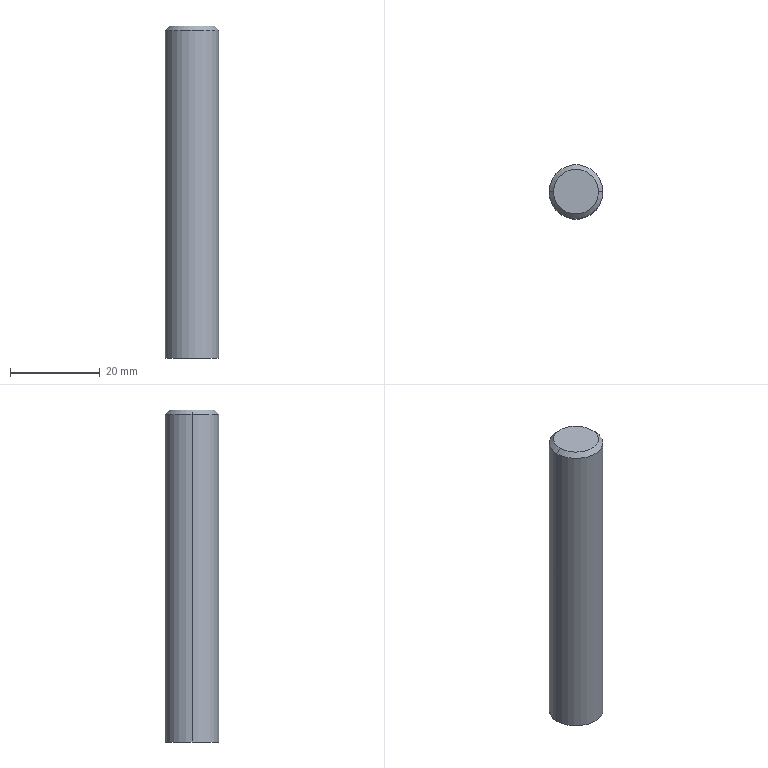Part | 1 solid | 15 faces | box 12 x 12 x 74 mm | volume 7564 mm3 | cone 6 | cylinder 6 | plane 3 | commonest cylinder face diameters 5 x2 8 x2 12 x2
STEP:
#1=CARTESIAN_POINT('',(2.5,0.,8.55));
#2=VERTEX_POINT('',#1);
#3=CARTESIAN_POINT('',(-2.5,0.,8.55));
#4=VERTEX_POINT('',#3);
#5=CARTESIAN_POINT('',(0.,0.,8.55));
#6=DIRECTION('',(0.,0.,-1.));
#7=DIRECTION('',(-1.,0.,0.));
#8=AXIS2_PLACEMENT_3D('',#5,#6,#7);
#9=CIRCLE('',#8,2.5);
#10=EDGE_CURVE('',#2,#4,#9,.T.);
#11=ORIENTED_EDGE('',*,*,#10,.F.);
#12=CARTESIAN_POINT('',(3.05,0.,8.));
#13=VERTEX_POINT('',#12);
#14=CARTESIAN_POINT('',(3.05,0.,8.));
#15=DIRECTION('',(0.7071,0.,-0.7071));
#16=VECTOR('',#15,1000.);
#17=LINE('',#14,#16);
#18=EDGE_CURVE('',#2,#13,#17,.T.);
#19=ORIENTED_EDGE('',*,*,#18,.T.);
#20=CARTESIAN_POINT('',(-3.05,0.,8.));
#21=VERTEX_POINT('',#20);
#22=CARTESIAN_POINT('',(0.,0.,8.));
#23=DIRECTION('',(0.,0.,-1.));
#24=DIRECTION('',(-1.,0.,0.));
#25=AXIS2_PLACEMENT_3D('',#22,#23,#24);
#26=CIRCLE('',#25,3.05);
#27=EDGE_CURVE('',#13,#21,#26,.T.);
#28=ORIENTED_EDGE('',*,*,#27,.T.);
#29=CARTESIAN_POINT('',(-3.05,0.,8.));
#30=DIRECTION('',(-0.7071,0.,-0.7071));
#31=VECTOR('',#30,1000.);
#32=LINE('',#29,#31);
#33=EDGE_CURVE('',#4,#21,#32,.T.);
#34=ORIENTED_EDGE('',*,*,#33,.F.);
#35=EDGE_LOOP('',(#11,#19,#28,#34));
#36=FACE_OUTER_BOUND('',#35,.T.);
#37=CARTESIAN_POINT('',(0.,0.,8.));
#38=DIRECTION('',(0.,0.,-1.));
#39=DIRECTION('',(-1.,0.,0.));
#40=AXIS2_PLACEMENT_3D('',#37,#38,#39);
#41=CONICAL_SURFACE('',#40,3.05,0.7854);
#42=ADVANCED_FACE('',(#36),#41,.F.);
#43=CARTESIAN_POINT('',(2.5,0.,27.));
#44=VERTEX_POINT('',#43);
#45=CARTESIAN_POINT('',(-2.5,0.,27.));
#46=VERTEX_POINT('',#45);
#47=CARTESIAN_POINT('',(0.,0.,27.));
#48=DIRECTION('',(0.,0.,-1.));
#49=DIRECTION('',(-1.,0.,0.));
#50=AXIS2_PLACEMENT_3D('',#47,#48,#49);
#51=CIRCLE('',#50,2.5);
#52=EDGE_CURVE('',#44,#46,#51,.T.);
#53=ORIENTED_EDGE('',*,*,#52,.F.);
#54=CARTESIAN_POINT('',(2.5,0.,8.));
#55=DIRECTION('',(0.,0.,-1.));
#56=VECTOR('',#55,1000.);
#57=LINE('',#54,#56);
#58=EDGE_CURVE('',#44,#2,#57,.T.);
#59=ORIENTED_EDGE('',*,*,#58,.T.);
#60=ORIENTED_EDGE('',*,*,#10,.T.);
#61=CARTESIAN_POINT('',(-2.5,0.,8.));
#62=DIRECTION('',(0.,0.,-1.));
#63=VECTOR('',#62,1000.);
#64=LINE('',#61,#63);
#65=EDGE_CURVE('',#46,#4,#64,.T.);
#66=ORIENTED_EDGE('',*,*,#65,.F.);
#67=EDGE_LOOP('',(#53,#59,#60,#66));
#68=FACE_OUTER_BOUND('',#67,.T.);
#69=CARTESIAN_POINT('',(0.,0.,8.));
#70=DIRECTION('',(0.,0.,-1.));
#71=DIRECTION('',(-1.,0.,0.));
#72=AXIS2_PLACEMENT_3D('',#69,#70,#71);
#73=CYLINDRICAL_SURFACE('',#72,2.5);
#74=ADVANCED_FACE('',(#68),#73,.F.);
#75=CARTESIAN_POINT('',(0.,0.,28.502));
#76=VERTEX_POINT('',#75);
#77=CARTESIAN_POINT('',(-2.5,0.,27.));
#78=DIRECTION('',(-0.8572,0.,-0.515));
#79=VECTOR('',#78,1000.);
#80=LINE('',#77,#79);
#81=EDGE_CURVE('',#76,#46,#80,.T.);
#82=ORIENTED_EDGE('',*,*,#81,.F.);
#83=CARTESIAN_POINT('',(2.5,0.,27.));
#84=DIRECTION('',(0.8572,0.,-0.515));
#85=VECTOR('',#84,1000.);
#86=LINE('',#83,#85);
#87=EDGE_CURVE('',#76,#44,#86,.T.);
#88=ORIENTED_EDGE('',*,*,#87,.T.);
#89=ORIENTED_EDGE('',*,*,#52,.T.);
#90=EDGE_LOOP('',(#82,#88,#89));
#91=FACE_OUTER_BOUND('',#90,.T.);
#92=CARTESIAN_POINT('',(0.,0.,27.));
#93=DIRECTION('',(0.,0.,-1.));
#94=DIRECTION('',(-1.,0.,0.));
#95=AXIS2_PLACEMENT_3D('',#92,#93,#94);
#96=CONICAL_SURFACE('',#95,2.5,1.03);
#97=ADVANCED_FACE('',(#91),#96,.F.);
#98=CARTESIAN_POINT('',(4.,0.,8.));
#99=VERTEX_POINT('',#98);
#100=CARTESIAN_POINT('',(-4.,0.,8.));
#101=VERTEX_POINT('',#100);
#102=CARTESIAN_POINT('',(0.,0.,8.));
#103=DIRECTION('',(0.,0.,-1.));
#104=DIRECTION('',(-1.,0.,0.));
#105=AXIS2_PLACEMENT_3D('',#102,#103,#104);
#106=CIRCLE('',#105,4.);
#107=EDGE_CURVE('',#99,#101,#106,.T.);
#108=ORIENTED_EDGE('',*,*,#107,.F.);
#109=CARTESIAN_POINT('',(4.,0.,0.));
#110=VERTEX_POINT('',#109);
#111=CARTESIAN_POINT('',(4.,0.,8.));
#112=DIRECTION('',(0.,0.,-1.));
#113=VECTOR('',#112,1000.);
#114=LINE('',#111,#113);
#115=EDGE_CURVE('',#99,#110,#114,.T.);
#116=ORIENTED_EDGE('',*,*,#115,.T.);
#117=CARTESIAN_POINT('',(-4.,0.,0.));
#118=VERTEX_POINT('',#117);
#119=CARTESIAN_POINT('',(0.,0.,0.));
#120=DIRECTION('',(0.,0.,-1.));
#121=DIRECTION('',(-1.,0.,0.));
#122=AXIS2_PLACEMENT_3D('',#119,#120,#121);
#123=CIRCLE('',#122,4.);
#124=EDGE_CURVE('',#110,#118,#123,.T.);
#125=ORIENTED_EDGE('',*,*,#124,.T.);
#126=CARTESIAN_POINT('',(-4.,0.,8.));
#127=DIRECTION('',(0.,0.,-1.));
#128=VECTOR('',#127,1000.);
#129=LINE('',#126,#128);
#130=EDGE_CURVE('',#101,#118,#129,.T.);
#131=ORIENTED_EDGE('',*,*,#130,.F.);
#132=EDGE_LOOP('',(#108,#116,#125,#131));
#133=FACE_OUTER_BOUND('',#132,.T.);
#134=CARTESIAN_POINT('',(0.,0.,8.));
#135=DIRECTION('',(0.,0.,-1.));
#136=DIRECTION('',(-1.,0.,0.));
#137=AXIS2_PLACEMENT_3D('',#134,#135,#136);
#138=CYLINDRICAL_SURFACE('',#137,4.);
#139=ADVANCED_FACE('',(#133),#138,.F.);
#140=CARTESIAN_POINT('',(5.,0.,74.));
#141=VERTEX_POINT('',#140);
#142=CARTESIAN_POINT('',(-5.,0.,74.));
#143=VERTEX_POINT('',#142);
#144=CARTESIAN_POINT('',(0.,0.,74.));
#145=DIRECTION('',(0.,0.,1.));
#146=DIRECTION('',(1.,0.,0.));
#147=AXIS2_PLACEMENT_3D('',#144,#145,#146);
#148=CIRCLE('',#147,5.);
#149=EDGE_CURVE('',#141,#143,#148,.T.);
#150=ORIENTED_EDGE('',*,*,#149,.F.);
#151=CARTESIAN_POINT('',(6.,0.,73.));
#152=VERTEX_POINT('',#151);
#153=CARTESIAN_POINT('',(5.,0.,74.));
#154=DIRECTION('',(0.7071,0.,-0.7071));
#155=VECTOR('',#154,1000.);
#156=LINE('',#153,#155);
#157=EDGE_CURVE('',#141,#152,#156,.T.);
#158=ORIENTED_EDGE('',*,*,#157,.T.);
#159=CARTESIAN_POINT('',(-6.,0.,73.));
#160=VERTEX_POINT('',#159);
#161=CARTESIAN_POINT('',(0.,0.,73.));
#162=DIRECTION('',(0.,0.,-1.));
#163=DIRECTION('',(1.,0.,0.));
#164=AXIS2_PLACEMENT_3D('',#161,#162,#163);
#165=CIRCLE('',#164,6.);
#166=EDGE_CURVE('',#160,#152,#165,.T.);
#167=ORIENTED_EDGE('',*,*,#166,.F.);
#168=CARTESIAN_POINT('',(-5.,0.,74.));
#169=DIRECTION('',(-0.7071,0.,-0.7071));
#170=VECTOR('',#169,1000.);
#171=LINE('',#168,#170);
#172=EDGE_CURVE('',#143,#160,#171,.T.);
#173=ORIENTED_EDGE('',*,*,#172,.F.);
#174=EDGE_LOOP('',(#150,#158,#167,#173));
#175=FACE_OUTER_BOUND('',#174,.T.);
#176=CARTESIAN_POINT('',(0.,0.,74.));
#177=DIRECTION('',(0.,0.,-1.));
#178=DIRECTION('',(-1.,0.,0.));
#179=AXIS2_PLACEMENT_3D('',#176,#177,#178);
#180=CONICAL_SURFACE('',#179,5.,0.7854);
#181=ADVANCED_FACE('',(#175),#180,.T.);
#182=ORIENTED_EDGE('',*,*,#166,.T.);
#183=CARTESIAN_POINT('',(6.,0.,0.));
#184=VERTEX_POINT('',#183);
#185=CARTESIAN_POINT('',(6.,0.,74.));
#186=DIRECTION('',(0.,0.,-1.));
#187=VECTOR('',#186,1000.);
#188=LINE('',#185,#187);
#189=EDGE_CURVE('',#152,#184,#188,.T.);
#190=ORIENTED_EDGE('',*,*,#189,.T.);
#191=CARTESIAN_POINT('',(-6.,0.,0.));
#192=VERTEX_POINT('',#191);
#193=CARTESIAN_POINT('',(0.,0.,0.));
#194=DIRECTION('',(0.,0.,1.));
#195=DIRECTION('',(1.,0.,0.));
#196=AXIS2_PLACEMENT_3D('',#193,#194,#195);
#197=CIRCLE('',#196,6.);
#198=EDGE_CURVE('',#184,#192,#197,.T.);
#199=ORIENTED_EDGE('',*,*,#198,.T.);
#200=CARTESIAN_POINT('',(-6.,0.,74.));
#201=DIRECTION('',(0.,0.,-1.));
#202=VECTOR('',#201,1000.);
#203=LINE('',#200,#202);
#204=EDGE_CURVE('',#160,#192,#203,.T.);
#205=ORIENTED_EDGE('',*,*,#204,.F.);
#206=EDGE_LOOP('',(#182,#190,#199,#205));
#207=FACE_OUTER_BOUND('',#206,.T.);
#208=CARTESIAN_POINT('',(0.,0.,74.));
#209=DIRECTION('',(0.,0.,-1.));
#210=DIRECTION('',(-1.,0.,0.));
#211=AXIS2_PLACEMENT_3D('',#208,#209,#210);
#212=CYLINDRICAL_SURFACE('',#211,6.);
#213=ADVANCED_FACE('',(#207),#212,.T.);
#214=ORIENTED_EDGE('',*,*,#189,.F.);
#215=CARTESIAN_POINT('',(0.,0.,73.));
#216=DIRECTION('',(0.,0.,-1.));
#217=DIRECTION('',(1.,0.,0.));
#218=AXIS2_PLACEMENT_3D('',#215,#216,#217);
#219=CIRCLE('',#218,6.);
#220=EDGE_CURVE('',#152,#160,#219,.T.);
#221=ORIENTED_EDGE('',*,*,#220,.T.);
#222=ORIENTED_EDGE('',*,*,#204,.T.);
#223=CARTESIAN_POINT('',(0.,0.,0.));
#224=DIRECTION('',(0.,0.,1.));
#225=DIRECTION('',(1.,0.,0.));
#226=AXIS2_PLACEMENT_3D('',#223,#224,#225);
#227=CIRCLE('',#226,6.);
#228=EDGE_CURVE('',#192,#184,#227,.T.);
#229=ORIENTED_EDGE('',*,*,#228,.T.);
#230=EDGE_LOOP('',(#214,#221,#222,#229));
#231=FACE_OUTER_BOUND('',#230,.T.);
#232=CARTESIAN_POINT('',(0.,0.,74.));
#233=DIRECTION('',(0.,0.,-1.));
#234=DIRECTION('',(-1.,0.,0.));
#235=AXIS2_PLACEMENT_3D('',#232,#233,#234);
#236=CYLINDRICAL_SURFACE('',#235,6.);
#237=ADVANCED_FACE('',(#231),#236,.T.);
#238=CARTESIAN_POINT('',(0.,0.,74.));
#239=DIRECTION('',(0.,0.,1.));
#240=DIRECTION('',(1.,0.,0.));
#241=AXIS2_PLACEMENT_3D('',#238,#239,#240);
#242=CIRCLE('',#241,5.);
#243=EDGE_CURVE('',#143,#141,#242,.T.);
#244=ORIENTED_EDGE('',*,*,#243,.T.);
#245=ORIENTED_EDGE('',*,*,#149,.T.);
#246=EDGE_LOOP('',(#244,#245));
#247=FACE_OUTER_BOUND('',#246,.T.);
#248=CARTESIAN_POINT('',(0.,0.,74.));
#249=DIRECTION('',(0.,0.,1.));
#250=DIRECTION('',(1.,0.,0.));
#251=AXIS2_PLACEMENT_3D('',#248,#249,#250);
#252=PLANE('',#251);
#253=ADVANCED_FACE('',(#247),#252,.T.);
#254=ORIENTED_EDGE('',*,*,#228,.F.);
#255=ORIENTED_EDGE('',*,*,#198,.F.);
#256=EDGE_LOOP('',(#254,#255));
#257=FACE_OUTER_BOUND('',#256,.T.);
#258=CARTESIAN_POINT('',(0.,0.,0.));
#259=DIRECTION('',(0.,0.,-1.));
#260=DIRECTION('',(-1.,0.,0.));
#261=AXIS2_PLACEMENT_3D('',#258,#259,#260);
#262=CIRCLE('',#261,4.);
#263=EDGE_CURVE('',#118,#110,#262,.T.);
#264=ORIENTED_EDGE('',*,*,#263,.F.);
#265=ORIENTED_EDGE('',*,*,#124,.F.);
#266=EDGE_LOOP('',(#264,#265));
#267=FACE_BOUND('',#266,.T.);
#268=CARTESIAN_POINT('',(0.,0.,0.));
#269=DIRECTION('',(0.,0.,1.));
#270=DIRECTION('',(1.,0.,0.));
#271=AXIS2_PLACEMENT_3D('',#268,#269,#270);
#272=PLANE('',#271);
#273=ADVANCED_FACE('',(#257,#267),#272,.F.);
#274=ORIENTED_EDGE('',*,*,#157,.F.);
#275=ORIENTED_EDGE('',*,*,#243,.F.);
#276=ORIENTED_EDGE('',*,*,#172,.T.);
#277=ORIENTED_EDGE('',*,*,#220,.F.);
#278=EDGE_LOOP('',(#274,#275,#276,#277));
#279=FACE_OUTER_BOUND('',#278,.T.);
#280=CARTESIAN_POINT('',(0.,0.,74.));
#281=DIRECTION('',(0.,0.,-1.));
#282=DIRECTION('',(-1.,0.,0.));
#283=AXIS2_PLACEMENT_3D('',#280,#281,#282);
#284=CONICAL_SURFACE('',#283,5.,0.7854);
#285=ADVANCED_FACE('',(#279),#284,.T.);
#286=ORIENTED_EDGE('',*,*,#115,.F.);
#287=CARTESIAN_POINT('',(0.,0.,8.));
#288=DIRECTION('',(0.,0.,-1.));
#289=DIRECTION('',(-1.,0.,0.));
#290=AXIS2_PLACEMENT_3D('',#287,#288,#289);
#291=CIRCLE('',#290,4.);
#292=EDGE_CURVE('',#101,#99,#291,.T.);
#293=ORIENTED_EDGE('',*,*,#292,.F.);
#294=ORIENTED_EDGE('',*,*,#130,.T.);
#295=ORIENTED_EDGE('',*,*,#263,.T.);
#296=EDGE_LOOP('',(#286,#293,#294,#295));
#297=FACE_OUTER_BOUND('',#296,.T.);
#298=CARTESIAN_POINT('',(0.,0.,8.));
#299=DIRECTION('',(0.,0.,-1.));
#300=DIRECTION('',(-1.,0.,0.));
#301=AXIS2_PLACEMENT_3D('',#298,#299,#300);
#302=CYLINDRICAL_SURFACE('',#301,4.);
#303=ADVANCED_FACE('',(#297),#302,.F.);
#304=ORIENTED_EDGE('',*,*,#292,.T.);
#305=ORIENTED_EDGE('',*,*,#107,.T.);
#306=EDGE_LOOP('',(#304,#305));
#307=FACE_OUTER_BOUND('',#306,.T.);
#308=CARTESIAN_POINT('',(0.,0.,8.));
#309=DIRECTION('',(0.,0.,-1.));
#310=DIRECTION('',(-1.,0.,0.));
#311=AXIS2_PLACEMENT_3D('',#308,#309,#310);
#312=CIRCLE('',#311,3.05);
#313=EDGE_CURVE('',#21,#13,#312,.T.);
#314=ORIENTED_EDGE('',*,*,#313,.F.);
#315=ORIENTED_EDGE('',*,*,#27,.F.);
#316=EDGE_LOOP('',(#314,#315));
#317=FACE_BOUND('',#316,.T.);
#318=CARTESIAN_POINT('',(0.,0.,8.));
#319=DIRECTION('',(0.,0.,-1.));
#320=DIRECTION('',(0.,-1.,0.));
#321=AXIS2_PLACEMENT_3D('',#318,#319,#320);
#322=PLANE('',#321);
#323=ADVANCED_FACE('',(#307,#317),#322,.T.);
#324=ORIENTED_EDGE('',*,*,#87,.F.);
#325=ORIENTED_EDGE('',*,*,#81,.T.);
#326=CARTESIAN_POINT('',(0.,0.,27.));
#327=DIRECTION('',(0.,0.,-1.));
#328=DIRECTION('',(-1.,0.,0.));
#329=AXIS2_PLACEMENT_3D('',#326,#327,#328);
#330=CIRCLE('',#329,2.5);
#331=EDGE_CURVE('',#46,#44,#330,.T.);
#332=ORIENTED_EDGE('',*,*,#331,.T.);
#333=EDGE_LOOP('',(#324,#325,#332));
#334=FACE_OUTER_BOUND('',#333,.T.);
#335=CARTESIAN_POINT('',(0.,0.,27.));
#336=DIRECTION('',(0.,0.,-1.));
#337=DIRECTION('',(-1.,0.,0.));
#338=AXIS2_PLACEMENT_3D('',#335,#336,#337);
#339=CONICAL_SURFACE('',#338,2.5,1.03);
#340=ADVANCED_FACE('',(#334),#339,.F.);
#341=ORIENTED_EDGE('',*,*,#58,.F.);
#342=ORIENTED_EDGE('',*,*,#331,.F.);
#343=ORIENTED_EDGE('',*,*,#65,.T.);
#344=CARTESIAN_POINT('',(0.,0.,8.55));
#345=DIRECTION('',(0.,0.,-1.));
#346=DIRECTION('',(-1.,0.,0.));
#347=AXIS2_PLACEMENT_3D('',#344,#345,#346);
#348=CIRCLE('',#347,2.5);
#349=EDGE_CURVE('',#4,#2,#348,.T.);
#350=ORIENTED_EDGE('',*,*,#349,.T.);
#351=EDGE_LOOP('',(#341,#342,#343,#350));
#352=FACE_OUTER_BOUND('',#351,.T.);
#353=CARTESIAN_POINT('',(0.,0.,8.));
#354=DIRECTION('',(0.,0.,-1.));
#355=DIRECTION('',(-1.,0.,0.));
#356=AXIS2_PLACEMENT_3D('',#353,#354,#355);
#357=CYLINDRICAL_SURFACE('',#356,2.5);
#358=ADVANCED_FACE('',(#352),#357,.F.);
#359=ORIENTED_EDGE('',*,*,#18,.F.);
#360=ORIENTED_EDGE('',*,*,#349,.F.);
#361=ORIENTED_EDGE('',*,*,#33,.T.);
#362=ORIENTED_EDGE('',*,*,#313,.T.);
#363=EDGE_LOOP('',(#359,#360,#361,#362));
#364=FACE_OUTER_BOUND('',#363,.T.);
#365=CARTESIAN_POINT('',(0.,0.,8.));
#366=DIRECTION('',(0.,0.,-1.));
#367=DIRECTION('',(-1.,0.,0.));
#368=AXIS2_PLACEMENT_3D('',#365,#366,#367);
#369=CONICAL_SURFACE('',#368,3.05,0.7854);
#370=ADVANCED_FACE('',(#364),#369,.F.);
#371=CLOSED_SHELL('',(#42,#74,#97,#139,#181,#213,#237,#253,#273,#285,#303,#323,#340,#358,#370));
#372=MANIFOLD_SOLID_BREP('',#371);
#373=CARTESIAN_POINT('',(0.,0.,0.));
#374=DIRECTION('',(0.,0.,1.));
#375=DIRECTION('',(1.,0.,0.));
#376=AXIS2_PLACEMENT_3D('',#373,#374,#375);
#377=(LENGTH_UNIT()NAMED_UNIT(*)SI_UNIT(.MILLI.,.METRE.));
#378=UNCERTAINTY_MEASURE_WITH_UNIT(LENGTH_MEASURE(0.00001),#377,'','');
#379=(NAMED_UNIT(*)PLANE_ANGLE_UNIT()SI_UNIT($,.RADIAN.));
#380=(NAMED_UNIT(*)SI_UNIT($,.STERADIAN.)SOLID_ANGLE_UNIT());
#381=(GEOMETRIC_REPRESENTATION_CONTEXT(3)GLOBAL_UNCERTAINTY_ASSIGNED_CONTEXT((#378))GLOBAL_UNIT_ASSIGNED_CONTEXT((#377,#379,#380))REPRESENTATION_CONTEXT('',''));
#382=ADVANCED_BREP_SHAPE_REPRESENTATION('',(#372,#376),#381);